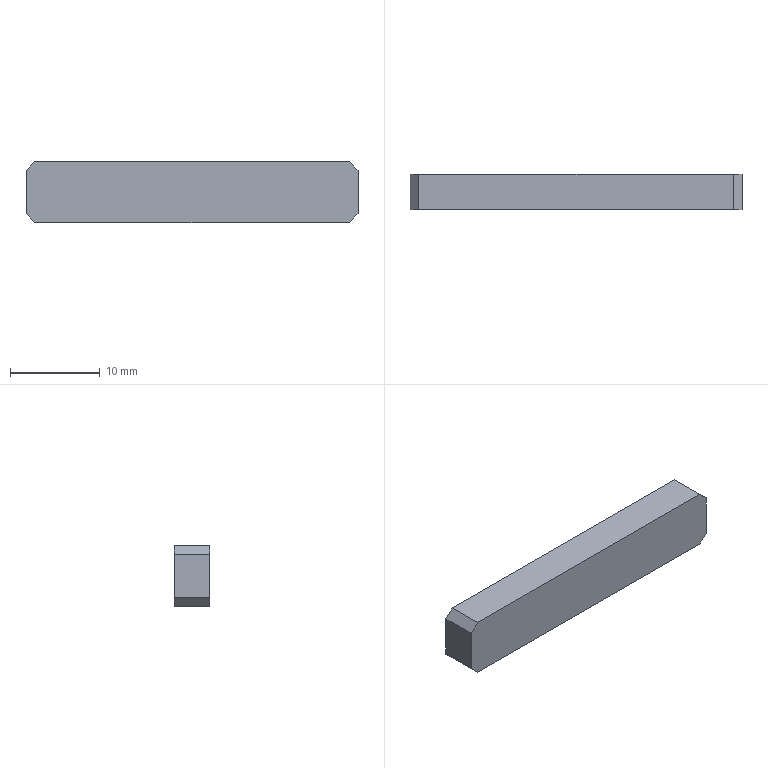Part | SolidWorks | features Chamfer 1, Extrusion 1 | 1 solid | 10 faces | box 37 x 4 x 6.8 mm | volume 998.4 mm3 | plane 10
STEP:
#1=CARTESIAN_POINT('',(18.5,-2.,2.4));
#2=VERTEX_POINT('',#1);
#3=CARTESIAN_POINT('',(18.5,-2.,-2.4));
#4=VERTEX_POINT('',#3);
#5=CARTESIAN_POINT('',(18.5,-2.,-3.4));
#6=DIRECTION('',(0.,0.,-1.));
#7=VECTOR('',#6,1000.);
#8=LINE('',#5,#7);
#9=EDGE_CURVE('',#2,#4,#8,.T.);
#10=ORIENTED_EDGE('',*,*,#9,.T.);
#11=CARTESIAN_POINT('',(18.5,2.,-2.4));
#12=VERTEX_POINT('',#11);
#13=CARTESIAN_POINT('',(18.5,2.,-2.4));
#14=DIRECTION('',(0.,1.,0.));
#15=VECTOR('',#14,1000.);
#16=LINE('',#13,#15);
#17=EDGE_CURVE('',#4,#12,#16,.T.);
#18=ORIENTED_EDGE('',*,*,#17,.T.);
#19=CARTESIAN_POINT('',(18.5,2.,2.4));
#20=VERTEX_POINT('',#19);
#21=CARTESIAN_POINT('',(18.5,2.,-3.4));
#22=DIRECTION('',(0.,0.,-1.));
#23=VECTOR('',#22,1000.);
#24=LINE('',#21,#23);
#25=EDGE_CURVE('',#20,#12,#24,.T.);
#26=ORIENTED_EDGE('',*,*,#25,.F.);
#27=CARTESIAN_POINT('',(18.5,2.,2.4));
#28=DIRECTION('',(0.,-1.,0.));
#29=VECTOR('',#28,1000.);
#30=LINE('',#27,#29);
#31=EDGE_CURVE('',#20,#2,#30,.T.);
#32=ORIENTED_EDGE('',*,*,#31,.T.);
#33=EDGE_LOOP('',(#10,#18,#26,#32));
#34=FACE_OUTER_BOUND('',#33,.T.);
#35=CARTESIAN_POINT('',(18.5,2.,-3.4));
#36=DIRECTION('',(-1.,0.,0.));
#37=DIRECTION('',(0.,0.,1.));
#38=AXIS2_PLACEMENT_3D('',#35,#36,#37);
#39=PLANE('',#38);
#40=ADVANCED_FACE('',(#34),#39,.F.);
#41=CARTESIAN_POINT('',(17.5,-2.,-3.4));
#42=VERTEX_POINT('',#41);
#43=CARTESIAN_POINT('',(-17.5,-2.,-3.4));
#44=VERTEX_POINT('',#43);
#45=CARTESIAN_POINT('',(-18.5,-2.,-3.4));
#46=DIRECTION('',(-1.,0.,0.));
#47=VECTOR('',#46,1000.);
#48=LINE('',#45,#47);
#49=EDGE_CURVE('',#42,#44,#48,.T.);
#50=ORIENTED_EDGE('',*,*,#49,.T.);
#51=CARTESIAN_POINT('',(-17.5,2.,-3.4));
#52=VERTEX_POINT('',#51);
#53=CARTESIAN_POINT('',(-17.5,2.,-3.4));
#54=DIRECTION('',(0.,1.,0.));
#55=VECTOR('',#54,1000.);
#56=LINE('',#53,#55);
#57=EDGE_CURVE('',#44,#52,#56,.T.);
#58=ORIENTED_EDGE('',*,*,#57,.T.);
#59=CARTESIAN_POINT('',(17.5,2.,-3.4));
#60=VERTEX_POINT('',#59);
#61=CARTESIAN_POINT('',(-18.5,2.,-3.4));
#62=DIRECTION('',(-1.,0.,0.));
#63=VECTOR('',#62,1000.);
#64=LINE('',#61,#63);
#65=EDGE_CURVE('',#60,#52,#64,.T.);
#66=ORIENTED_EDGE('',*,*,#65,.F.);
#67=CARTESIAN_POINT('',(17.5,2.,-3.4));
#68=DIRECTION('',(0.,-1.,0.));
#69=VECTOR('',#68,1000.);
#70=LINE('',#67,#69);
#71=EDGE_CURVE('',#60,#42,#70,.T.);
#72=ORIENTED_EDGE('',*,*,#71,.T.);
#73=EDGE_LOOP('',(#50,#58,#66,#72));
#74=FACE_OUTER_BOUND('',#73,.T.);
#75=CARTESIAN_POINT('',(-18.5,2.,-3.4));
#76=DIRECTION('',(0.,0.,1.));
#77=DIRECTION('',(1.,0.,0.));
#78=AXIS2_PLACEMENT_3D('',#75,#76,#77);
#79=PLANE('',#78);
#80=ADVANCED_FACE('',(#74),#79,.F.);
#81=CARTESIAN_POINT('',(-18.5,2.,-2.4));
#82=VERTEX_POINT('',#81);
#83=CARTESIAN_POINT('',(-18.5,2.,2.4));
#84=VERTEX_POINT('',#83);
#85=CARTESIAN_POINT('',(-18.5,2.,-3.4));
#86=DIRECTION('',(0.,0.,1.));
#87=VECTOR('',#86,1000.);
#88=LINE('',#85,#87);
#89=EDGE_CURVE('',#82,#84,#88,.T.);
#90=ORIENTED_EDGE('',*,*,#89,.F.);
#91=CARTESIAN_POINT('',(-18.5,-2.,-2.4));
#92=VERTEX_POINT('',#91);
#93=CARTESIAN_POINT('',(-18.5,2.,-2.4));
#94=DIRECTION('',(0.,-1.,0.));
#95=VECTOR('',#94,1000.);
#96=LINE('',#93,#95);
#97=EDGE_CURVE('',#82,#92,#96,.T.);
#98=ORIENTED_EDGE('',*,*,#97,.T.);
#99=CARTESIAN_POINT('',(-18.5,-2.,2.4));
#100=VERTEX_POINT('',#99);
#101=CARTESIAN_POINT('',(-18.5,-2.,-3.4));
#102=DIRECTION('',(0.,0.,1.));
#103=VECTOR('',#102,1000.);
#104=LINE('',#101,#103);
#105=EDGE_CURVE('',#92,#100,#104,.T.);
#106=ORIENTED_EDGE('',*,*,#105,.T.);
#107=CARTESIAN_POINT('',(-18.5,2.,2.4));
#108=DIRECTION('',(0.,1.,0.));
#109=VECTOR('',#108,1000.);
#110=LINE('',#107,#109);
#111=EDGE_CURVE('',#100,#84,#110,.T.);
#112=ORIENTED_EDGE('',*,*,#111,.T.);
#113=EDGE_LOOP('',(#90,#98,#106,#112));
#114=FACE_OUTER_BOUND('',#113,.T.);
#115=CARTESIAN_POINT('',(-18.5,2.,-3.4));
#116=DIRECTION('',(1.,0.,0.));
#117=DIRECTION('',(0.,0.,-1.));
#118=AXIS2_PLACEMENT_3D('',#115,#116,#117);
#119=PLANE('',#118);
#120=ADVANCED_FACE('',(#114),#119,.F.);
#121=CARTESIAN_POINT('',(-17.5,2.,3.4));
#122=VERTEX_POINT('',#121);
#123=CARTESIAN_POINT('',(17.5,2.,3.4));
#124=VERTEX_POINT('',#123);
#125=CARTESIAN_POINT('',(-18.5,2.,3.4));
#126=DIRECTION('',(1.,0.,0.));
#127=VECTOR('',#126,1000.);
#128=LINE('',#125,#127);
#129=EDGE_CURVE('',#122,#124,#128,.T.);
#130=ORIENTED_EDGE('',*,*,#129,.F.);
#131=CARTESIAN_POINT('',(-17.5,-2.,3.4));
#132=VERTEX_POINT('',#131);
#133=CARTESIAN_POINT('',(-17.5,2.,3.4));
#134=DIRECTION('',(0.,-1.,0.));
#135=VECTOR('',#134,1000.);
#136=LINE('',#133,#135);
#137=EDGE_CURVE('',#122,#132,#136,.T.);
#138=ORIENTED_EDGE('',*,*,#137,.T.);
#139=CARTESIAN_POINT('',(17.5,-2.,3.4));
#140=VERTEX_POINT('',#139);
#141=CARTESIAN_POINT('',(-18.5,-2.,3.4));
#142=DIRECTION('',(1.,0.,0.));
#143=VECTOR('',#142,1000.);
#144=LINE('',#141,#143);
#145=EDGE_CURVE('',#132,#140,#144,.T.);
#146=ORIENTED_EDGE('',*,*,#145,.T.);
#147=CARTESIAN_POINT('',(17.5,2.,3.4));
#148=DIRECTION('',(0.,1.,0.));
#149=VECTOR('',#148,1000.);
#150=LINE('',#147,#149);
#151=EDGE_CURVE('',#140,#124,#150,.T.);
#152=ORIENTED_EDGE('',*,*,#151,.T.);
#153=EDGE_LOOP('',(#130,#138,#146,#152));
#154=FACE_OUTER_BOUND('',#153,.T.);
#155=CARTESIAN_POINT('',(-18.5,2.,3.4));
#156=DIRECTION('',(0.,0.,-1.));
#157=DIRECTION('',(-1.,0.,0.));
#158=AXIS2_PLACEMENT_3D('',#155,#156,#157);
#159=PLANE('',#158);
#160=ADVANCED_FACE('',(#154),#159,.F.);
#161=ORIENTED_EDGE('',*,*,#65,.T.);
#162=CARTESIAN_POINT('',(-10.45,2.,-10.45));
#163=DIRECTION('',(-0.7071,0.,0.7071));
#164=VECTOR('',#163,1000.);
#165=LINE('',#162,#164);
#166=EDGE_CURVE('',#52,#82,#165,.T.);
#167=ORIENTED_EDGE('',*,*,#166,.T.);
#168=ORIENTED_EDGE('',*,*,#89,.T.);
#169=CARTESIAN_POINT('',(-10.45,2.,10.45));
#170=DIRECTION('',(0.7071,0.,0.7071));
#171=VECTOR('',#170,1000.);
#172=LINE('',#169,#171);
#173=EDGE_CURVE('',#84,#122,#172,.T.);
#174=ORIENTED_EDGE('',*,*,#173,.T.);
#175=ORIENTED_EDGE('',*,*,#129,.T.);
#176=CARTESIAN_POINT('',(10.45,2.,10.45));
#177=DIRECTION('',(0.7071,0.,-0.7071));
#178=VECTOR('',#177,1000.);
#179=LINE('',#176,#178);
#180=EDGE_CURVE('',#124,#20,#179,.T.);
#181=ORIENTED_EDGE('',*,*,#180,.T.);
#182=ORIENTED_EDGE('',*,*,#25,.T.);
#183=CARTESIAN_POINT('',(10.45,2.,-10.45));
#184=DIRECTION('',(-0.7071,0.,-0.7071));
#185=VECTOR('',#184,1000.);
#186=LINE('',#183,#185);
#187=EDGE_CURVE('',#12,#60,#186,.T.);
#188=ORIENTED_EDGE('',*,*,#187,.T.);
#189=EDGE_LOOP('',(#161,#167,#168,#174,#175,#181,#182,#188));
#190=FACE_OUTER_BOUND('',#189,.T.);
#191=CARTESIAN_POINT('',(0.,2.,0.));
#192=DIRECTION('',(0.,1.,0.));
#193=DIRECTION('',(0.,0.,1.));
#194=AXIS2_PLACEMENT_3D('',#191,#192,#193);
#195=PLANE('',#194);
#196=ADVANCED_FACE('',(#190),#195,.T.);
#197=ORIENTED_EDGE('',*,*,#105,.F.);
#198=CARTESIAN_POINT('',(-18.5,-2.,-2.4));
#199=DIRECTION('',(0.7071,0.,-0.7071));
#200=VECTOR('',#199,1000.);
#201=LINE('',#198,#200);
#202=EDGE_CURVE('',#92,#44,#201,.T.);
#203=ORIENTED_EDGE('',*,*,#202,.T.);
#204=ORIENTED_EDGE('',*,*,#49,.F.);
#205=CARTESIAN_POINT('',(17.5,-2.,-3.4));
#206=DIRECTION('',(0.7071,0.,0.7071));
#207=VECTOR('',#206,1000.);
#208=LINE('',#205,#207);
#209=EDGE_CURVE('',#42,#4,#208,.T.);
#210=ORIENTED_EDGE('',*,*,#209,.T.);
#211=ORIENTED_EDGE('',*,*,#9,.F.);
#212=CARTESIAN_POINT('',(18.5,-2.,2.4));
#213=DIRECTION('',(-0.7071,0.,0.7071));
#214=VECTOR('',#213,1000.);
#215=LINE('',#212,#214);
#216=EDGE_CURVE('',#2,#140,#215,.T.);
#217=ORIENTED_EDGE('',*,*,#216,.T.);
#218=ORIENTED_EDGE('',*,*,#145,.F.);
#219=CARTESIAN_POINT('',(-17.5,-2.,3.4));
#220=DIRECTION('',(-0.7071,0.,-0.7071));
#221=VECTOR('',#220,1000.);
#222=LINE('',#219,#221);
#223=EDGE_CURVE('',#132,#100,#222,.T.);
#224=ORIENTED_EDGE('',*,*,#223,.T.);
#225=EDGE_LOOP('',(#197,#203,#204,#210,#211,#217,#218,#224));
#226=FACE_OUTER_BOUND('',#225,.T.);
#227=CARTESIAN_POINT('',(0.,-2.,0.));
#228=DIRECTION('',(0.,1.,0.));
#229=DIRECTION('',(0.,0.,1.));
#230=AXIS2_PLACEMENT_3D('',#227,#228,#229);
#231=PLANE('',#230);
#232=ADVANCED_FACE('',(#226),#231,.F.);
#233=ORIENTED_EDGE('',*,*,#166,.F.);
#234=ORIENTED_EDGE('',*,*,#57,.F.);
#235=ORIENTED_EDGE('',*,*,#202,.F.);
#236=ORIENTED_EDGE('',*,*,#97,.F.);
#237=EDGE_LOOP('',(#233,#234,#235,#236));
#238=FACE_OUTER_BOUND('',#237,.T.);
#239=CARTESIAN_POINT('',(-18.5,2.,-2.4));
#240=DIRECTION('',(0.7071,0.,0.7071));
#241=DIRECTION('',(0.,-1.,0.));
#242=AXIS2_PLACEMENT_3D('',#239,#240,#241);
#243=PLANE('',#242);
#244=ADVANCED_FACE('',(#238),#243,.F.);
#245=ORIENTED_EDGE('',*,*,#173,.F.);
#246=ORIENTED_EDGE('',*,*,#111,.F.);
#247=ORIENTED_EDGE('',*,*,#223,.F.);
#248=ORIENTED_EDGE('',*,*,#137,.F.);
#249=EDGE_LOOP('',(#245,#246,#247,#248));
#250=FACE_OUTER_BOUND('',#249,.T.);
#251=CARTESIAN_POINT('',(-17.5,2.,3.4));
#252=DIRECTION('',(0.7071,0.,-0.7071));
#253=DIRECTION('',(0.,-1.,0.));
#254=AXIS2_PLACEMENT_3D('',#251,#252,#253);
#255=PLANE('',#254);
#256=ADVANCED_FACE('',(#250),#255,.F.);
#257=ORIENTED_EDGE('',*,*,#187,.F.);
#258=ORIENTED_EDGE('',*,*,#17,.F.);
#259=ORIENTED_EDGE('',*,*,#209,.F.);
#260=ORIENTED_EDGE('',*,*,#71,.F.);
#261=EDGE_LOOP('',(#257,#258,#259,#260));
#262=FACE_OUTER_BOUND('',#261,.T.);
#263=CARTESIAN_POINT('',(17.5,2.,-3.4));
#264=DIRECTION('',(-0.7071,0.,0.7071));
#265=DIRECTION('',(0.,-1.,0.));
#266=AXIS2_PLACEMENT_3D('',#263,#264,#265);
#267=PLANE('',#266);
#268=ADVANCED_FACE('',(#262),#267,.F.);
#269=ORIENTED_EDGE('',*,*,#180,.F.);
#270=ORIENTED_EDGE('',*,*,#151,.F.);
#271=ORIENTED_EDGE('',*,*,#216,.F.);
#272=ORIENTED_EDGE('',*,*,#31,.F.);
#273=EDGE_LOOP('',(#269,#270,#271,#272));
#274=FACE_OUTER_BOUND('',#273,.T.);
#275=CARTESIAN_POINT('',(18.5,2.,2.4));
#276=DIRECTION('',(-0.7071,0.,-0.7071));
#277=DIRECTION('',(0.,-1.,0.));
#278=AXIS2_PLACEMENT_3D('',#275,#276,#277);
#279=PLANE('',#278);
#280=ADVANCED_FACE('',(#274),#279,.F.);
#281=CLOSED_SHELL('',(#40,#80,#120,#160,#196,#232,#244,#256,#268,#280));
#282=MANIFOLD_SOLID_BREP('',#281);
#283=CARTESIAN_POINT('',(0.,0.,0.));
#284=DIRECTION('',(0.,0.,1.));
#285=DIRECTION('',(1.,0.,0.));
#286=AXIS2_PLACEMENT_3D('',#283,#284,#285);
#287=(LENGTH_UNIT()NAMED_UNIT(*)SI_UNIT(.MILLI.,.METRE.));
#288=UNCERTAINTY_MEASURE_WITH_UNIT(LENGTH_MEASURE(0.00001),#287,'','');
#289=(NAMED_UNIT(*)PLANE_ANGLE_UNIT()SI_UNIT($,.RADIAN.));
#290=(NAMED_UNIT(*)SI_UNIT($,.STERADIAN.)SOLID_ANGLE_UNIT());
#291=(GEOMETRIC_REPRESENTATION_CONTEXT(3)GLOBAL_UNCERTAINTY_ASSIGNED_CONTEXT((#288))GLOBAL_UNIT_ASSIGNED_CONTEXT((#287,#289,#290))REPRESENTATION_CONTEXT('',''));
#292=ADVANCED_BREP_SHAPE_REPRESENTATION('',(#282,#286),#291);